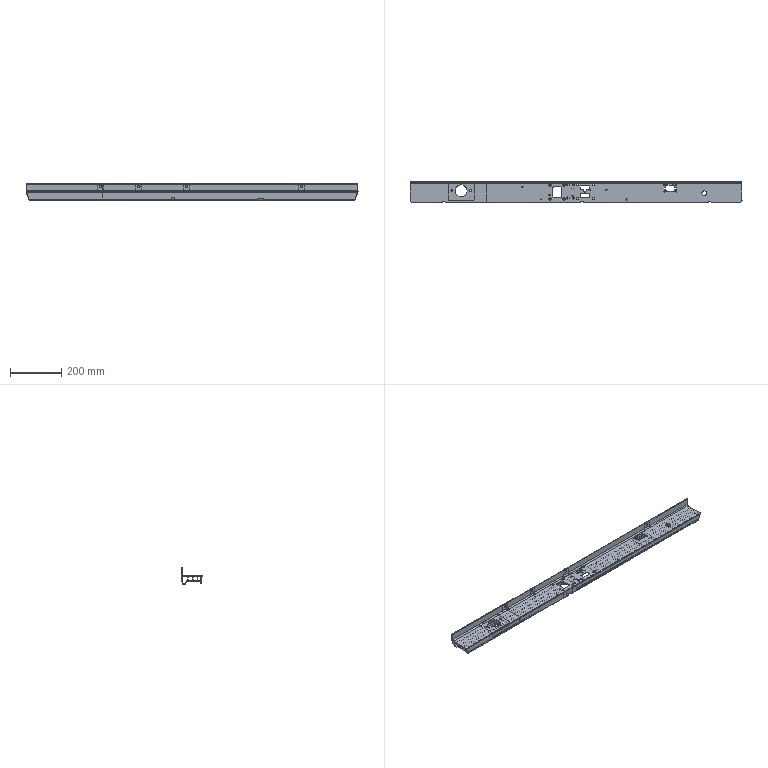NC program | NX | posted with a generic post | part box 1301 x 81.1 x 63 mm
Lines 6765 to 7608 of 19815:
(ZLEVEL_PROFILE_1_COPY_1 , TOOL : D8R0.5)
N13522 T08 M6
N13524 G54
N13526 G17 G0 G90 X1132.802 Y56.359 B0. C0. S6000 M3
N13528 G43 Z30. H8
N13530 Z1.408
N13532 G94 G1 Z-0.092 F1000.
N13534 X1132.535 Y55.178
N13536 G3 X1132.772 Y54.414 R0.8
N13538 G1 X1142.175 Y45.72 F2500.
N13540 G2 X1143.454 Y42.796 R3.983
N13542 G1 Y-30.296
N13544 G2 X1142.174 Y-33.221 R3.982
N13546 G1 X1133.521 Y-41.214
N13548 X1133.511 Y-41.26 Z-0.185
N13550 X1142.211 Y-33.222
N13552 G3 X1143.492 Y-30.294 R3.986
N13554 G1 Y42.795
N13556 G3 X1142.213 Y45.721 R3.985
N13558 G1 X1132.783 Y54.439
N13560 X1132.794 Y54.464 Z-0.277
N13562 X1142.251 Y45.721
N13564 G2 X1143.531 Y42.795 R3.985
N13566 G1 Y-30.296
N13568 G2 X1142.25 Y-33.221 R3.983
N13570 G1 X1133.551 Y-41.258
N13572 X1133.503 Y-41.3
N13574 X1133.495 Y-41.34 Z-0.37
N13576 X1133.59 Y-41.258
N13578 X1142.288 Y-33.222
N13580 G3 X1143.569 Y-30.295 R3.985
N13582 G1 Y42.8
N13584 G3 X1142.286 Y45.724 R3.983
N13586 G1 X1141.669 Y46.294
N13588 X1132.805 Y54.49
N13590 X1132.813 Y54.5 Z-0.416
N13592 X1132.821 Y54.511 Z-0.462
N13594 X1141.462 Y46.521
N13596 X1142.324 Y45.724
N13598 G2 X1143.607 Y42.8 R3.983
N13600 G1 Y-30.295
N13602 G2 X1142.327 Y-33.221 R3.984
N13604 G1 X1133.608 Y-41.277
N13606 X1133.488 Y-41.382
N13608 X1133.481 Y-41.423 Z-0.554
N13610 X1133.608 Y-41.312
N13612 X1142.365 Y-33.222
N13614 G3 X1143.646 Y-30.295 R3.985
N13616 G1 Y42.8
N13618 G3 X1142.362 Y45.724 R3.983
N13620 G1 X1141.397 Y46.616
N13622 X1132.841 Y54.527
N13624 X1132.851 Y54.536 Z-0.601
N13626 X1132.861 Y54.544 Z-0.647
N13628 X1132.902 Y54.507
N13630 X1141.371 Y46.675
N13632 X1142.4 Y45.724
N13634 G2 X1143.684 Y42.8 R3.983
N13636 G1 Y-30.295
N13638 G2 X1142.403 Y-33.222 R3.986
N13640 G1 X1133.608 Y-41.347
N13642 X1133.474 Y-41.465
N13644 X1133.468 Y-41.507 Z-0.739
N13646 X1133.608 Y-41.383
N13648 X1142.442 Y-33.221
N13650 G3 X1143.722 Y-30.296 R3.983
N13652 G1 Y42.8
N13654 G3 X1142.439 Y45.724 R3.983
N13656 G1 X1141.373 Y46.709
N13658 X1132.881 Y54.56
N13660 X1132.892 Y54.569 Z-0.785
N13662 X1132.901 Y54.576 Z-0.831
N13664 X1141.396 Y46.723
N13666 X1142.477 Y45.724
N13668 G2 X1143.76 Y42.8 R3.983
N13670 G1 Y-30.295
N13672 G2 X1142.48 Y-33.222 R3.985
N13674 G1 X1133.608 Y-41.418
N13676 X1133.461 Y-41.549
N13678 X1133.455 Y-41.591 Z-0.924
N13680 X1133.608 Y-41.453
N13682 X1142.517 Y-33.222
N13684 G3 X1143.799 Y-30.294 R3.986
N13686 G1 Y42.8
N13688 G3 X1142.515 Y45.724 R3.983
N13690 G1 X1141.433 Y46.724
N13692 X1132.921 Y54.593
N13694 X1132.933 Y54.602 Z-0.97
N13696 X1132.941 Y54.609 Z-1.016
N13698 X1141.471 Y46.724
N13700 X1142.554 Y45.724
N13702 G2 X1143.837 Y42.8 R3.983
N13704 G1 Y-30.295
N13706 G2 X1142.556 Y-33.222 R3.985
N13708 G1 X1133.449 Y-41.634
N13710 X1133.448 Y-41.671 Z-1.109
N13712 X1142.594 Y-33.222
N13714 G3 X1143.875 Y-30.295 R3.985
N13716 G1 Y42.8
N13718 G3 X1142.592 Y45.724 R3.983
N13720 G1 X1141.509 Y46.724
N13722 X1133.093 Y54.507
N13724 X1132.961 Y54.625
N13726 X1132.973 Y54.635 Z-1.155
N13728 X1132.982 Y54.642 Z-1.201
N13730 X1133.131 Y54.507
N13732 X1141.548 Y46.724
N13734 X1142.63 Y45.724
N13736 G2 X1143.913 Y42.8 R3.99
N13738 G1 Y-30.295
N13740 G2 X1142.632 Y-33.222 R3.986
N13742 G1 X1133.502 Y-41.657
N13744 X1133.451 Y-41.701
N13746 X1133.455 Y-41.731 Z-1.293
N13748 X1133.54 Y-41.657
N13750 X1142.671 Y-33.222
N13752 G3 X1143.952 Y-30.295 R3.985
N13754 G1 Y42.8
N13756 G3 X1142.668 Y45.724 R4.013
N13758 G1 X1141.586 Y46.724
N13760 X1133.17 Y54.507
N13762 X1133.002 Y54.658
N13764 X1133.014 Y54.668 Z-1.34
N13766 X1133.022 Y54.674 Z-1.386
N13768 X1133.208 Y54.507
N13770 X1141.624 Y46.724
N13772 X1142.707 Y45.724
N13774 G2 X1143.99 Y42.8 R4.034
N13776 G1 Y-30.295
N13778 G2 X1142.709 Y-33.222 R3.984
N13780 G1 X1133.579 Y-41.657
N13782 X1133.458 Y-41.762
N13784 X1133.463 Y-41.793 Z-1.478
N13786 X1133.608 Y-41.665
N13788 X1142.748 Y-33.221
N13790 G3 X1144.028 Y-30.296 R3.983
N13792 G1 Y42.829
N13794 G3 X1143.63 Y44.531 R3.838
N13796 X1142.745 Y45.724 R4.169
N13798 G1 X1141.662 Y46.724
N13800 X1133.209 Y54.542
N13802 X1133.042 Y54.691
N13804 X1133.055 Y54.701 Z-1.524
N13806 X1133.063 Y54.708 Z-1.571
N13808 X1133.209 Y54.577
N13810 X1141.701 Y46.724
N13812 X1142.783 Y45.724
N13814 G2 X1143.372 Y45.04 R4.36
N13816 X1144.067 Y42.824 R3.885
N13818 G1 Y-30.294
N13820 G2 X1142.785 Y-33.222 R3.987
N13822 G1 X1133.608 Y-41.701
N13824 X1133.467 Y-41.824
N13826 X1133.472 Y-41.856 Z-1.663
N13828 X1133.608 Y-41.736
N13830 X1142.824 Y-33.222
N13832 G3 X1144.105 Y-30.294 R3.986
N13834 G1 Y42.822
N13836 G3 X1143.4 Y45.055 R3.89
N13838 X1142.821 Y45.724 R4.365
N13840 G1 X1141.739 Y46.724
N13842 X1133.209 Y54.612
N13844 X1133.083 Y54.725
N13846 X1133.095 Y54.735 Z-1.709
N13848 X1133.104 Y54.742 Z-1.755
N13850 X1141.777 Y46.724
N13852 X1142.86 Y45.724
N13854 G2 X1143.431 Y45.065 R4.36
N13856 X1144.143 Y42.82 R3.896
N13858 G1 Y-30.296
N13860 G2 X1142.863 Y-33.221 R3.983
N13862 G1 X1133.608 Y-41.771
N13864 X1133.476 Y-41.887
N13866 X1133.481 Y-41.919 Z-1.848
N13868 X1133.608 Y-41.807
N13870 X1142.901 Y-33.222
N13872 G3 X1144.181 Y-30.295 R3.984
N13874 G1 Y42.8
N13876 G3 X1143.602 Y44.861 R3.95
N13878 X1142.898 Y45.724 R4.227
N13880 G1 X1141.815 Y46.724
N13882 X1133.125 Y54.758
N13884 X1133.136 Y54.768 Z-1.894
N13886 X1133.145 Y54.775 Z-1.94
N13888 X1141.854 Y46.724
N13890 X1142.936 Y45.724
N13892 G2 X1144.002 Y44.093 R4.078
N13894 X1144.22 Y42.8 R3.928
N13896 G1 Y-30.294
N13898 G2 X1142.938 Y-33.222 R3.987
N13900 G1 X1133.608 Y-41.842
N13902 X1133.486 Y-41.95
N13904 X1133.491 Y-41.982 Z-2.033
N13906 X1133.608 Y-41.878
N13908 X1142.978 Y-33.221
N13910 G3 X1144.258 Y-30.296 R3.983
N13912 G1 Y42.8
N13914 G3 X1142.974 Y45.724 R3.983
N13916 G1 X1141.892 Y46.724
N13918 X1133.166 Y54.792
N13920 X1133.177 Y54.801 Z-2.079
N13922 X1133.186 Y54.809 Z-2.125
N13924 X1141.93 Y46.724
N13926 X1143.013 Y45.724
N13928 G2 X1144.296 Y42.8 R3.983
N13930 G1 Y-30.294
N13932 G2 X1143.015 Y-33.223 R3.986
N13934 G1 X1133.496 Y-42.014
N13936 X1133.501 Y-42.046 Z-2.217
N13938 X1143.054 Y-33.222
N13940 G3 X1144.334 Y-30.295 R3.984
N13942 G1 Y42.8
N13944 G3 X1143.051 Y45.724 R3.99
N13946 G1 X1141.969 Y46.724
N13948 X1134.848 Y53.31
N13950 X1133.207 Y54.826
N13952 X1133.236 Y54.834 Z-2.31
N13954 X1142.007 Y46.724
N13956 X1143.089 Y45.724
N13958 G2 X1144.373 Y42.8 R4.011
N13960 G1 Y-30.294
N13962 G2 X1143.091 Y-33.223 R3.986
N13964 G1 X1133.509 Y-42.074
N13966 X1133.517 Y-42.1 Z-2.402
N13968 X1133.568 Y-42.057
N13970 X1143.13 Y-33.222
N13972 G3 X1144.411 Y-30.295 R3.985
N13974 G1 Y42.8
N13976 G3 X1143.128 Y45.724 R4.03
N13978 G1 X1142.045 Y46.724
N13980 X1133.608 Y54.526
N13982 X1133.266 Y54.841
N13984 X1133.296 Y54.849 Z-2.494
N13986 X1133.608 Y54.562
N13988 X1142.083 Y46.724
N13990 X1143.166 Y45.724
N13992 G2 X1144.219 Y44.132 R4.104
N13994 X1144.449 Y42.826 R3.813
N13996 G1 Y-30.294
N13998 G2 X1143.168 Y-33.222 R3.987
N14000 G1 X1133.606 Y-42.057
N14002 X1133.525 Y-42.126
N14004 X1133.534 Y-42.153 Z-2.587
N14006 X1133.608 Y-42.09
N14008 X1143.206 Y-33.223
N14010 G3 X1144.487 Y-30.294 R3.987
N14012 G1 Y42.829
N14014 G3 X1144.09 Y44.531 R3.839
N14016 X1143.204 Y45.724 R4.168
N14018 G1 X1142.122 Y46.724
N14020 X1133.608 Y54.597
N14022 X1133.326 Y54.856
N14024 X1133.357 Y54.864 Z-2.679
N14026 X1135.04 Y53.31
N14028 X1142.16 Y46.724
N14030 X1143.242 Y45.724
N14032 G2 X1144.104 Y44.579 R4.17
N14034 X1144.526 Y42.825 R3.855
N14036 G1 Y-30.295
N14038 G2 X1143.245 Y-33.221 R3.984
N14040 G1 X1133.608 Y-42.125
N14042 X1133.543 Y-42.18
N14044 X1133.553 Y-42.208 Z-2.772
N14046 X1133.608 Y-42.16
N14048 X1143.283 Y-33.222
N14050 G3 X1144.564 Y-30.295 R3.985
N14052 G1 Y42.827
N14054 G3 X1144.333 Y44.132 R3.812
N14056 X1143.281 Y45.724 R4.104
N14058 G1 X1142.198 Y46.724
N14060 X1135.078 Y53.31
N14062 X1133.387 Y54.872
N14064 X1133.417 Y54.879 Z-2.864
N14066 X1135.116 Y53.31
N14068 X1142.236 Y46.724
N14070 X1143.319 Y45.724
N14072 G2 X1144.602 Y42.8 R4.02
N14074 G1 Y-30.294
N14076 G2 X1143.321 Y-33.223 R3.986
N14078 G1 X1133.562 Y-42.235
N14080 X1133.571 Y-42.263 Z-2.956
N14082 X1143.36 Y-33.222
N14084 G3 X1144.641 Y-30.295 R3.984
N14086 G1 Y42.8
N14088 G3 X1143.357 Y45.724 R3.983
N14090 G1 X1142.275 Y46.724
N14092 X1135.155 Y53.31
N14094 X1133.447 Y54.887
N14096 X1133.477 Y54.894 Z-3.049
N14098 X1142.313 Y46.724
N14100 X1143.395 Y45.724
N14102 G2 X1144.679 Y42.8 R3.983
N14104 G1 Y-30.295
N14106 G2 X1143.398 Y-33.222 R3.984
N14108 G1 X1133.581 Y-42.29
N14110 X1133.59 Y-42.317 Z-3.141
N14112 X1143.436 Y-33.222
N14114 G3 X1144.717 Y-30.295 R3.985
N14116 G1 Y42.8
N14118 G3 X1143.434 Y45.724 R3.997
N14120 G1 X1142.351 Y46.724
N14122 X1133.508 Y54.902
N14124 X1133.539 Y54.908 Z-3.234
N14126 X1142.39 Y46.724
N14128 X1143.472 Y45.724
N14130 G2 X1144.755 Y42.8 R4.02
N14132 G1 Y-30.295
N14134 G2 X1143.474 Y-33.222 R3.985
N14136 G1 X1133.599 Y-42.345
N14138 X1133.609 Y-42.372 Z-3.326
N14140 X1143.513 Y-33.221
N14142 G3 X1144.794 Y-30.296 R3.983
N14144 G1 Y42.821
N14146 G3 X1144.401 Y44.519 R3.869
N14148 X1143.51 Y45.724 R4.133
N14150 G1 X1142.428 Y46.724
N14152 X1133.572 Y54.913
N14154 X1133.605 Y54.918 Z-3.418
N14156 X1142.466 Y46.724
N14158 X1143.548 Y45.724
N14160 G2 X1144.434 Y44.531 R4.189
N14162 X1144.832 Y42.833 R3.824
N14164 G1 Y28.023
N14166 Y-30.298
N14168 G2 X1143.561 Y-33.212 R3.976
N14170 G1 X1143.357 Y-33.402
N14172 X1142.656 Y-34.049
N14174 X1133.623 Y-42.394
N14176 X1133.631 Y-42.405 Z-3.465
N14178 X1133.638 Y-42.416 Z-3.511
N14180 X1142.483 Y-34.244
N14182 X1143.593 Y-33.219
N14184 G3 X1144.87 Y-30.299 R3.975
N14186 G1 Y27.97
N14188 Y42.824
N14190 G3 X1144.175 Y45.042 R3.883
N14192 X1143.587 Y45.724 R4.37
N14194 G1 X1142.504 Y46.724
N14196 X1133.639 Y54.922
N14198 X1133.673 Y54.926 Z-3.603
N14200 X1133.695 Y54.906
N14202 X1142.543 Y46.724
N14204 X1143.625 Y45.724
N14206 X1143.665 Y45.686
N14208 X1143.998 Y45.329
N14210 G2 X1144.908 Y42.8 R3.978
N14212 G1 Y-30.228
N14214 G2 X1143.625 Y-33.224 R3.988
N14216 G1 X1142.382 Y-34.373
N14218 X1133.653 Y-42.438
N14220 X1133.66 Y-42.448 Z-3.649
N14222 X1133.668 Y-42.459 Z-3.696
N14224 X1142.317 Y-34.468
N14226 X1143.663 Y-33.224
N14228 G3 X1144.947 Y-30.256 R4.034
N14230 G1 Y42.8
N14232 G3 X1144.037 Y45.329 R3.981
N14234 G1 X1144.002 Y45.371
N14236 X1143.663 Y45.724
N14238 X1142.581 Y46.724
N14240 X1135.031 Y53.709
N14242 X1133.706 Y54.93
N14244 X1133.74 Y54.934 Z-3.788
N14246 X1135.069 Y53.709
N14248 X1142.619 Y46.724
N14250 X1143.702 Y45.724
N14252 G2 X1144.275 Y45.062 R4.336
N14254 X1144.985 Y42.819 R3.9
N14256 G1 Y-30.284
N14258 G2 X1143.702 Y-33.224 R4.001
N14260 G1 X1142.277 Y-34.541
N14262 X1133.686 Y-42.476
N14264 X1133.696 Y-42.486 Z-3.834
N14266 X1133.705 Y-42.494 Z-3.88
N14268 X1142.252 Y-34.599
N14270 X1143.74 Y-33.224
N14272 G3 X1145.023 Y-30.3 R3.983
N14274 G1 Y42.826
N14276 G3 X1144.793 Y44.132 R3.816
N14278 X1143.74 Y45.724 R4.101
N14280 G1 X1142.657 Y46.724
N14282 X1135.108 Y53.709
N14284 X1133.774 Y54.938
N14286 X1133.807 Y54.942 Z-3.973
N14288 X1142.696 Y46.724
N14290 X1143.778 Y45.724
N14292 G2 X1145.061 Y42.8 R3.989
N14294 G1 Y-30.3
N14296 G2 X1143.778 Y-33.224 R3.983
N14298 G1 X1142.241 Y-34.644
N14300 X1133.723 Y-42.512
N14302 X1133.734 Y-42.522 Z-4.019
N14304 X1133.741 Y-42.529 Z-4.065
N14306 X1133.825 Y-42.456
N14308 X1143.802 Y-33.237
N14310 G3 X1145.1 Y-30.3 R4.005
N14312 G1 Y42.8
N14314 G3 X1143.816 Y45.724 R3.983
N14316 G1 X1142.734 Y46.724
N14318 X1133.841 Y54.946
N14320 X1133.874 Y54.949 Z-4.157
N14322 X1133.926 Y54.906
N14324 X1142.772 Y46.724
N14326 X1143.855 Y45.724
N14328 G2 X1145.138 Y42.8 R3.997
N14330 G1 Y-30.3
N14332 G2 X1143.855 Y-33.224 R3.983
N14334 G1 X1133.863 Y-42.456
N14336 X1133.76 Y-42.547
N14338 X1133.771 Y-42.558 Z-4.204
N14340 X1133.778 Y-42.565 Z-4.25
N14342 X1133.901 Y-42.456
N14344 X1143.893 Y-33.224
N14346 G3 X1145.176 Y-30.3 R4.002
N14348 G1 Y42.8
N14350 G3 X1143.893 Y45.724 R4.018
N14352 G1 X1142.81 Y46.724
N14354 X1133.964 Y54.906
N14356 X1133.908 Y54.953
N14358 X1133.941 Y54.957 Z-4.342
N14360 X1134.002 Y54.906
N14362 X1142.849 Y46.724
N14364 X1143.931 Y45.724
N14366 G2 X1145.103 Y43.733 R4.067
N14368 X1145.215 Y42.824 R3.762
N14370 G1 Y-30.3
N14372 G2 X1143.931 Y-33.224 R4.02
N14374 G1 X1133.939 Y-42.456
N14376 X1133.797 Y-42.582
N14378 X1133.809 Y-42.594 Z-4.388
N14380 X1133.815 Y-42.6 Z-4.435
N14382 X1133.978 Y-42.456
N14384 X1143.969 Y-33.224
N14386 G3 X1145.253 Y-30.3 R4.034
N14388 G1 Y42.829
N14390 G3 X1144.855 Y44.531 R3.842
N14392 X1143.969 Y45.724 R4.164
N14394 G1 X1142.887 Y46.724
N14396 X1134.008 Y54.936
N14398 X1133.976 Y54.962
N14400 X1134.011 Y54.968 Z-4.527
N14402 X1135.377 Y53.709
N14404 X1142.925 Y46.724
N14406 X1144.008 Y45.724
N14408 G2 X1144.778 Y44.749 R4.208
N14410 X1145.291 Y42.822 R3.877
N14412 G1 Y-30.3
N14414 G2 X1144.339 Y-32.879 R3.982
N14416 G1 X1144.028 Y-33.206
N14418 X1142.384 Y-34.724
N14420 X1134.008 Y-42.463
N14422 X1133.833 Y-42.618
N14424 X1133.846 Y-42.63 Z-4.573
N14426 X1133.852 Y-42.636 Z-4.619
N14428 X1134.008 Y-42.498
N14430 X1142.422 Y-34.724
N14432 X1144.066 Y-33.205
N14434 X1144.378 Y-32.879
N14436 G3 X1145.329 Y-30.3 R3.978
N14438 G1 Y42.828
N14440 G3 X1144.906 Y44.583 R3.846
N14442 X1144.046 Y45.724 R4.188
N14444 G1 X1142.964 Y46.724
N14446 X1135.416 Y53.709
N14448 X1134.045 Y54.972
N14450 X1134.078 Y54.976 Z-4.712
N14452 G2 X1143.002 Y46.724 R2835.828
N14454 G1 X1144.084 Y45.724
N14456 G2 X1144.97 Y44.531 R4.161
N14458 X1145.368 Y42.828 R3.844
N14460 G1 Y-30.3
N14462 G2 X1144.084 Y-33.224 R4.035
N14464 G1 X1134.008 Y-42.534
N14466 X1133.871 Y-42.655
N14468 X1133.883 Y-42.666 Z-4.758
N14470 X1133.89 Y-42.673 Z-4.804
N14472 X1134.008 Y-42.569
N14474 X1144.123 Y-33.224
N14476 G3 X1145.406 Y-30.3 R4.009
N14478 G1 Y42.8
N14480 G3 X1144.123 Y45.724 R4.027
N14482 G1 X1143.04 Y46.724
N14484 G3 X1134.112 Y54.98 R6652.972
N14486 G1 X1134.146 Y54.984 Z-4.897
N14488 G2 X1143.078 Y46.724 R5151.952
N14490 G1 X1144.161 Y45.724
N14492 G2 X1145.444 Y42.8 R3.983
N14494 G1 Y-30.3
N14496 G2 X1144.161 Y-33.224 R3.983
N14498 G1 X1134.008 Y-42.604
N14500 X1133.909 Y-42.691
N14502 X1133.921 Y-42.702 Z-4.943
N14504 X1133.928 Y-42.71 Z-4.989
N14506 X1134.008 Y-42.64
N14508 X1144.199 Y-33.224
N14510 G3 X1145.482 Y-30.3 R3.983
N14512 G1 Y42.8
N14514 G3 X1144.199 Y45.724 R3.983
N14516 G1 X1143.117 Y46.724
N14518 G3 X1134.179 Y54.988 R2252.66
N14520 G1 X1134.212 Y54.991 Z-5.081
N14522 G2 X1143.155 Y46.724 R2035.11
N14524 G1 X1144.237 Y45.724
N14526 G2 X1145.521 Y42.8 R4.005
N14528 G1 Y-30.3
N14530 G2 X1144.237 Y-33.224 R3.995
N14532 G1 X1142.614 Y-34.724
N14534 X1133.948 Y-42.728
N14536 X1133.958 Y-42.739 Z-5.128
N14538 X1133.967 Y-42.747 Z-5.174
N14540 X1142.652 Y-34.724
N14542 X1144.276 Y-33.224
N14544 G3 X1145.559 Y-30.3 R4.018
N14546 G1 Y42.8
N14548 G3 X1144.276 Y45.724 R4.028
N14550 G1 X1143.193 Y46.724
N14552 G3 X1134.246 Y54.995 R1785.712
N14554 G1 X1134.279 Y54.998 Z-5.266
N14556 G2 X1143.231 Y46.724 R1593.87
N14558 G1 X1144.314 Y45.724
N14560 G2 X1144.94 Y44.986 R4.328
N14562 X1145.597 Y42.828 R3.871
N14564 G1 Y-30.303
N14566 G2 X1144.507 Y-33.028 R3.951
N14568 X1144.314 Y-33.224 R8.555
N14570 G1 X1142.69 Y-34.724
N14572 X1133.986 Y-42.765
N14574 X1133.996 Y-42.775 Z-5.312
N14576 X1134.005 Y-42.784 Z-5.359
N14578 X1142.728 Y-34.724
N14580 X1144.352 Y-33.224
N14582 X1144.684 Y-32.879
N14584 G3 X1145.636 Y-30.3 R3.98
N14586 G1 Y42.825
N14588 G3 X1144.94 Y45.042 R3.881
N14590 X1144.352 Y45.724 R4.382
N14592 G1 X1143.27 Y46.724
N14594 G3 X1134.313 Y55.002 R1519.966
N14596 G1 X1134.348 Y55.008 Z-5.451
N14598 G2 X1143.308 Y46.724 R1543.635
N14600 G1 X1144.39 Y45.724
N14602 X1144.45 Y45.667
N14604 X1144.764 Y45.329
N14606 X1144.801 Y45.281
N14608 G2 X1145.674 Y42.8 R3.964
N14610 G1 Y-30.303
N14612 G2 X1144.591 Y-33.017 R3.943
N14614 G1 X1144.43 Y-33.187
N14616 X1144.39 Y-33.224
N14618 X1142.767 Y-34.724
N14620 X1134.03 Y-42.796
N14622 X1134.056 Y-42.807 Z-5.543
N14624 X1142.805 Y-34.724
N14626 X1144.449 Y-33.206
N14628 X1144.76 Y-32.879
N14630 G3 X1145.712 Y-30.3 R3.981
N14632 G1 Y42.8
N14634 G3 X1144.801 Y45.33 R3.978
N14636 G1 X1144.469 Y45.686
N14638 X1144.429 Y45.724
N14640 X1143.346 Y46.724
N14642 G3 X1134.383 Y55.013 R1640.169
N14644 G1 X1134.418 Y55.019 Z-5.636
N14646 G2 X1143.384 Y46.724 R1622.092
N14648 G1 X1144.467 Y45.724
N14650 X1144.801 Y45.376
N14652 X1144.84 Y45.329
N14654 G2 X1145.75 Y42.8 R3.98
N14656 G1 Y-30.3
N14658 G2 X1144.799 Y-32.879 R3.981
N14660 G1 X1144.467 Y-33.224
N14662 X1142.843 Y-34.724
N14664 X1134.082 Y-42.819
N14666 X1134.108 Y-42.83 Z-5.728
N14668 X1142.882 Y-34.724
N14670 X1144.505 Y-33.224
N14672 X1144.674 Y-33.05
N14674 G3 X1145.789 Y-30.305 R3.939
N14676 G1 Y42.802
N14678 G3 X1144.815 Y45.403 R3.96
N14680 G1 X1144.505 Y45.724
N14682 X1143.423 Y46.724
N14684 G3 X1134.451 Y55.022 R1450.224
N14686 G1 X1134.484 Y55.026 Z-5.82
N14688 G2 X1143.461 Y46.724 R1396.411
N14690 G1 X1144.543 Y45.724
N14692 G2 X1145.429 Y44.531 R4.164
N14694 X1145.827 Y42.829 R3.842
N14696 G1 Y-30.306
N14698 G2 X1144.695 Y-33.07 R3.943
N14700 G1 X1144.543 Y-33.224
N14702 X1142.92 Y-34.724
N14704 X1134.134 Y-42.841
N14706 X1134.16 Y-42.853 Z-5.913
N14708 X1142.958 Y-34.724
N14710 X1144.582 Y-33.224
N14712 G3 X1145.865 Y-30.3 R3.988
N14714 G1 Y42.8
N14716 G3 X1144.582 Y45.724 R3.999
N14718 G1 X1143.499 Y46.724
N14720 X1142.42 Y47.724
N14722 X1141.991 Y48.123
N14724 X1141.603 Y48.489
N14726 G3 X1134.518 Y55.03 R1028.655
N14728 G1 X1134.551 Y55.034 Z-6.005
N14730 G2 X1141.607 Y48.522 R936.353
N14732 G1 X1142.03 Y48.123
N14734 X1142.458 Y47.724
N14736 X1143.538 Y46.724
N14738 X1144.62 Y45.724
N14740 G2 X1145.903 Y42.8 R3.983
N14742 G1 Y-30.3
N14744 G2 X1144.62 Y-33.224 R3.983
N14746 G1 X1142.996 Y-34.724
N14748 X1134.191 Y-42.859
N14750 X1134.222 Y-42.865 Z-6.098
N14752 X1143.035 Y-34.724
N14754 X1144.658 Y-33.224
N14756 G3 X1145.942 Y-30.3 R3.989
N14758 G1 Y42.8
N14760 G3 X1144.658 Y45.724 R4.004
N14762 G1 X1143.576 Y46.724
N14764 X1141.603 Y48.562
N14766 X1140.404 Y49.685
N14768 X1134.736 Y54.906
N14770 X1134.585 Y55.038
N14772 X1134.619 Y55.042 Z-6.19
N14774 X1134.775 Y54.906
N14776 X1140.407 Y49.719
N14778 X1141.603 Y48.598
N14780 X1143.614 Y46.724
N14782 X1144.697 Y45.724
N14784 G2 X1145.98 Y42.8 R4.025
N14786 G1 Y-30.3
N14788 G2 X1144.697 Y-33.224 R4.009
N14790 G1 X1143.073 Y-34.724
N14792 X1134.253 Y-42.871
N14794 X1134.284 Y-42.877 Z-6.282
N14796 X1143.111 Y-34.724
N14798 X1144.735 Y-33.224
N14800 G3 X1146.018 Y-30.3 R4.027
N14802 G1 Y42.826
N14804 G3 X1145.62 Y44.531 R3.855
N14806 X1144.735 Y45.724 R4.146
N14808 G1 X1143.652 Y46.724
N14810 X1141.203 Y49.007
N14812 X1140.871 Y49.32
N14814 X1140.804 Y49.385
N14816 X1134.808 Y54.912
N14818 X1134.653 Y55.046
N14820 X1134.687 Y55.051 Z-6.375
N14822 X1134.808 Y54.947
N14824 X1140.804 Y49.423
N14826 X1141.203 Y49.045
N14828 X1143.602 Y46.807
N14830 X1143.691 Y46.724
N14832 X1144.773 Y45.724
N14834 G2 X1145.659 Y44.531 R4.183
N14836 X1146.056 Y42.832 R3.829
N14838 G1 Y-30.303
N14840 G2 X1144.97 Y-33.021 R3.941
N14842 G1 X1144.801 Y-33.198
N14844 X1144.773 Y-33.224
N14846 X1143.149 Y-34.724
N14848 X1134.316 Y-42.883
N14850 X1134.347 Y-42.888 Z-6.467
N14852 X1134.388 Y-42.855
N14854 X1143.188 Y-34.724
N14856 X1144.831 Y-33.206
N14858 X1145.143 Y-32.879
N14860 G3 X1146.095 Y-30.3 R3.983
N14862 G1 Y42.822
N14864 G3 X1145.403 Y45.036 R3.89
N14866 X1144.811 Y45.724 R4.332
N14868 G1 X1143.729 Y46.724
N14870 X1141.373 Y48.921
N14872 X1140.804 Y49.461
N14874 X1134.808 Y54.983
N14876 X1134.722 Y55.056
N14878 X1134.757 Y55.062 Z-6.56
N14880 X1135.367 Y54.507
N14882 X1140.57 Y49.719
N14884 X1140.804 Y49.499
N14886 X1140.989 Y49.32
N14888 G3 X1143.767 Y46.724 R348.189
N14890 G1 X1144.85 Y45.724
N14892 G2 X1145.431 Y45.052 R4.33
N14894 X1146.133 Y42.82 R3.897
N14896 G1 Y-30.3
N14898 G2 X1145.181 Y-32.879 R3.978
N14900 G1 X1144.869 Y-33.205
N14902 X1143.226 Y-34.724
N14904 X1134.379 Y-42.895
N14906 X1134.412 Y-42.903 Z-6.652
N14908 X1143.264 Y-34.724
N14910 X1144.888 Y-33.224
N14912 X1144.947 Y-33.166
N14914 X1145.08 Y-33.026
N14916 G3 X1146.171 Y-30.307 R3.934
N14918 G1 Y42.826
N14920 G3 X1145.749 Y44.58 R3.851
N14922 X1144.888 Y45.724 R4.178
N14924 G1 X1143.805 Y46.724
N14926 G2 X1141.029 Y49.32 R332.401
N14928 G1 X1140.804 Y49.537
N14930 X1140.611 Y49.719
N14932 X1135.406 Y54.507
N14934 X1134.793 Y55.067
N14936 X1134.827 Y55.072 Z-6.744
N14938 X1135.445 Y54.507
N14940 X1140.651 Y49.719
N14942 X1140.804 Y49.575
N14944 X1141.068 Y49.32
N14946 G3 X1143.844 Y46.724 R316.304
N14948 G1 X1144.926 Y45.724
N14950 G2 X1146.21 Y42.8 R4.033
N14952 G1 Y-30.3
N14954 G2 X1144.926 Y-33.224 R4.014
N14956 G1 X1143.303 Y-34.724
N14958 X1134.446 Y-42.906
N14960 X1134.48 Y-42.909 Z-6.837
N14962 X1143.341 Y-34.724
N14964 X1144.964 Y-33.224
N14966 G3 X1146.248 Y-30.3 R3.983
N14968 G1 Y42.8
N14970 G3 X1144.964 Y45.724 R3.983
N14972 G1 X1143.882 Y46.724
N14974 G2 X1140.804 Y49.614 R226.273
N14976 G1 X1135.048 Y54.906
N14978 X1134.86 Y55.076
N14980 X1134.893 Y55.08 Z-6.929
N14982 X1135.087 Y54.906
N14984 X1140.804 Y49.652
N14986 G3 X1143.92 Y46.724 R219.885
N14988 G1 X1145.003 Y45.724
N14990 G2 X1146.286 Y42.8 R3.983
N14992 G1 Y-30.3
N14994 G2 X1145.003 Y-33.224 R3.983
N14996 G1 X1143.379 Y-34.724
N14998 X1134.514 Y-42.912
N15000 X1134.549 Y-42.916 Z-7.021
N15002 X1143.417 Y-34.724
N15004 X1145.041 Y-33.224
N15006 G3 X1146.324 Y-30.3 R4.002
N15008 G1 Y42.8
N15010 G3 X1145.041 Y45.724 R3.983
N15012 G1 X1143.959 Y46.724
N15014 G2 X1140.804 Y49.69 R221.183
N15016 G1 X1135.127 Y54.906
N15018 X1134.927 Y55.084
N15020 X1134.961 Y55.088 Z-7.114
N15022 X1135.166 Y54.906
N15024 X1140.814 Y49.719
N15026 G3 X1143.997 Y46.724 R226.056
N15028 G1 X1145.079 Y45.724
N15030 G2 X1146.363 Y42.8 R3.983
N15032 G1 Y-30.3
N15034 G2 X1145.079 Y-33.224 R4.025
N15036 G1 X1143.456 Y-34.724
N15038 X1134.583 Y-42.919
N15040 X1134.617 Y-42.922 Z-7.206
N15042 X1134.694 Y-42.855
N15044 X1145.117 Y-33.224
N15046 G3 X1145.31 Y-33.028 R9.225
N15048 X1146.401 Y-30.303 R3.949
N15050 G1 Y42.8
N15052 G3 X1145.117 Y45.724 R3.983
N15054 G1 X1144.035 Y46.724
N15056 G2 X1140.804 Y49.765 R246.14
N15058 G1 X1135.205 Y54.906
N15060 X1134.995 Y55.092
N15062 X1135.029 Y55.097 Z-7.299
N15064 X1135.207 Y54.94
N15066 X1140.404 Y50.17
N15068 G2 X1141.312 Y49.32 R5.626
N15070 G3 X1144.073 Y46.724 R242.708
N15072 G1 X1145.156 Y45.724
N15074 G2 X1146.439 Y42.8 R3.983
N15076 G1 Y-30.3
N15078 G2 X1145.487 Y-32.879 R3.98
N15080 G1 X1145.156 Y-33.224
N15082 X1134.732 Y-42.855
N15084 X1134.651 Y-42.925
N15086 X1134.685 Y-42.928 Z-7.391
N15088 X1134.77 Y-42.855
N15090 X1143.57 Y-34.724
N15092 X1145.214 Y-33.206
N15094 X1145.526 Y-32.879
N15096 G3 X1146.477 Y-30.3 R3.981
N15098 G1 Y42.8
N15100 G3 X1145.194 Y45.724 R3.983
N15102 G1 X1144.112 Y46.724
N15104 G2 X1141.821 Y48.869 R405.31
N15106 X1141.4 Y49.332 R4.188
N15108 G3 X1140.57 Y50.118 R3.887
N15110 G1 X1140.404 Y50.23
N15112 G2 X1140.015 Y50.563 R7.402
N15114 G1 X1135.207 Y54.977
N15116 X1135.064 Y55.102
N15118 X1135.099 Y55.108 Z-7.483
N15120 X1135.326 Y54.906
N15122 X1140.004 Y50.611
N15124 G3 X1140.404 Y50.326 R2.568
N15126 G2 X1141.504 Y49.32 R4.025
N15128 G1 X1141.808 Y48.921
N15130 G3 X1144.15 Y46.724 R339.739
N15132 G1 X1145.232 Y45.724
N15134 G2 X1146.516 Y42.8 R3.983
N15136 G1 Y-30.304
N15138 G2 X1145.434 Y-33.016 R3.94
N15140 G1 X1145.281 Y-33.177
N15142 X1145.232 Y-33.224
N15144 X1134.808 Y-42.856
N15146 X1134.719 Y-42.931
N15148 X1134.754 Y-42.936 Z-7.576
N15150 X1134.808 Y-42.891
N15152 X1145.271 Y-33.224
N15154 X1145.601 Y-32.881
N15156 G3 X1146.554 Y-30.3 R3.981
N15158 G1 Y42.8
N15160 G3 X1145.271 Y45.724 R3.983
N15162 G1 X1144.188 Y46.724
N15164 G2 X1142.003 Y48.774 R333.861
N15166 G1 X1141.864 Y48.921
N15168 X1141.597 Y49.32
N15170 G3 X1140.404 Y50.421 R4.078
N15172 G2 X1139.463 Y51.145 R6.809
N15174 G1 X1135.367 Y54.906
N15176 X1135.135 Y55.114
N15178 X1135.17 Y55.12 Z-7.668
N15180 X1135.607 Y54.724
N15182 X1139.205 Y51.419
N15184 X1139.318 Y51.315
N15186 X1139.604 Y51.094
N15188 X1140.749 Y50.281
N15190 G2 X1141.758 Y49.207 R3.73
N15192 G1 X1142.003 Y48.812
N15194 G3 X1144.226 Y46.724 R330.794
N15196 G1 X1145.309 Y45.724
N15198 G2 X1146.592 Y42.8 R3.983
N15200 G1 Y-30.305
N15202 G2 X1145.477 Y-33.052 R3.939